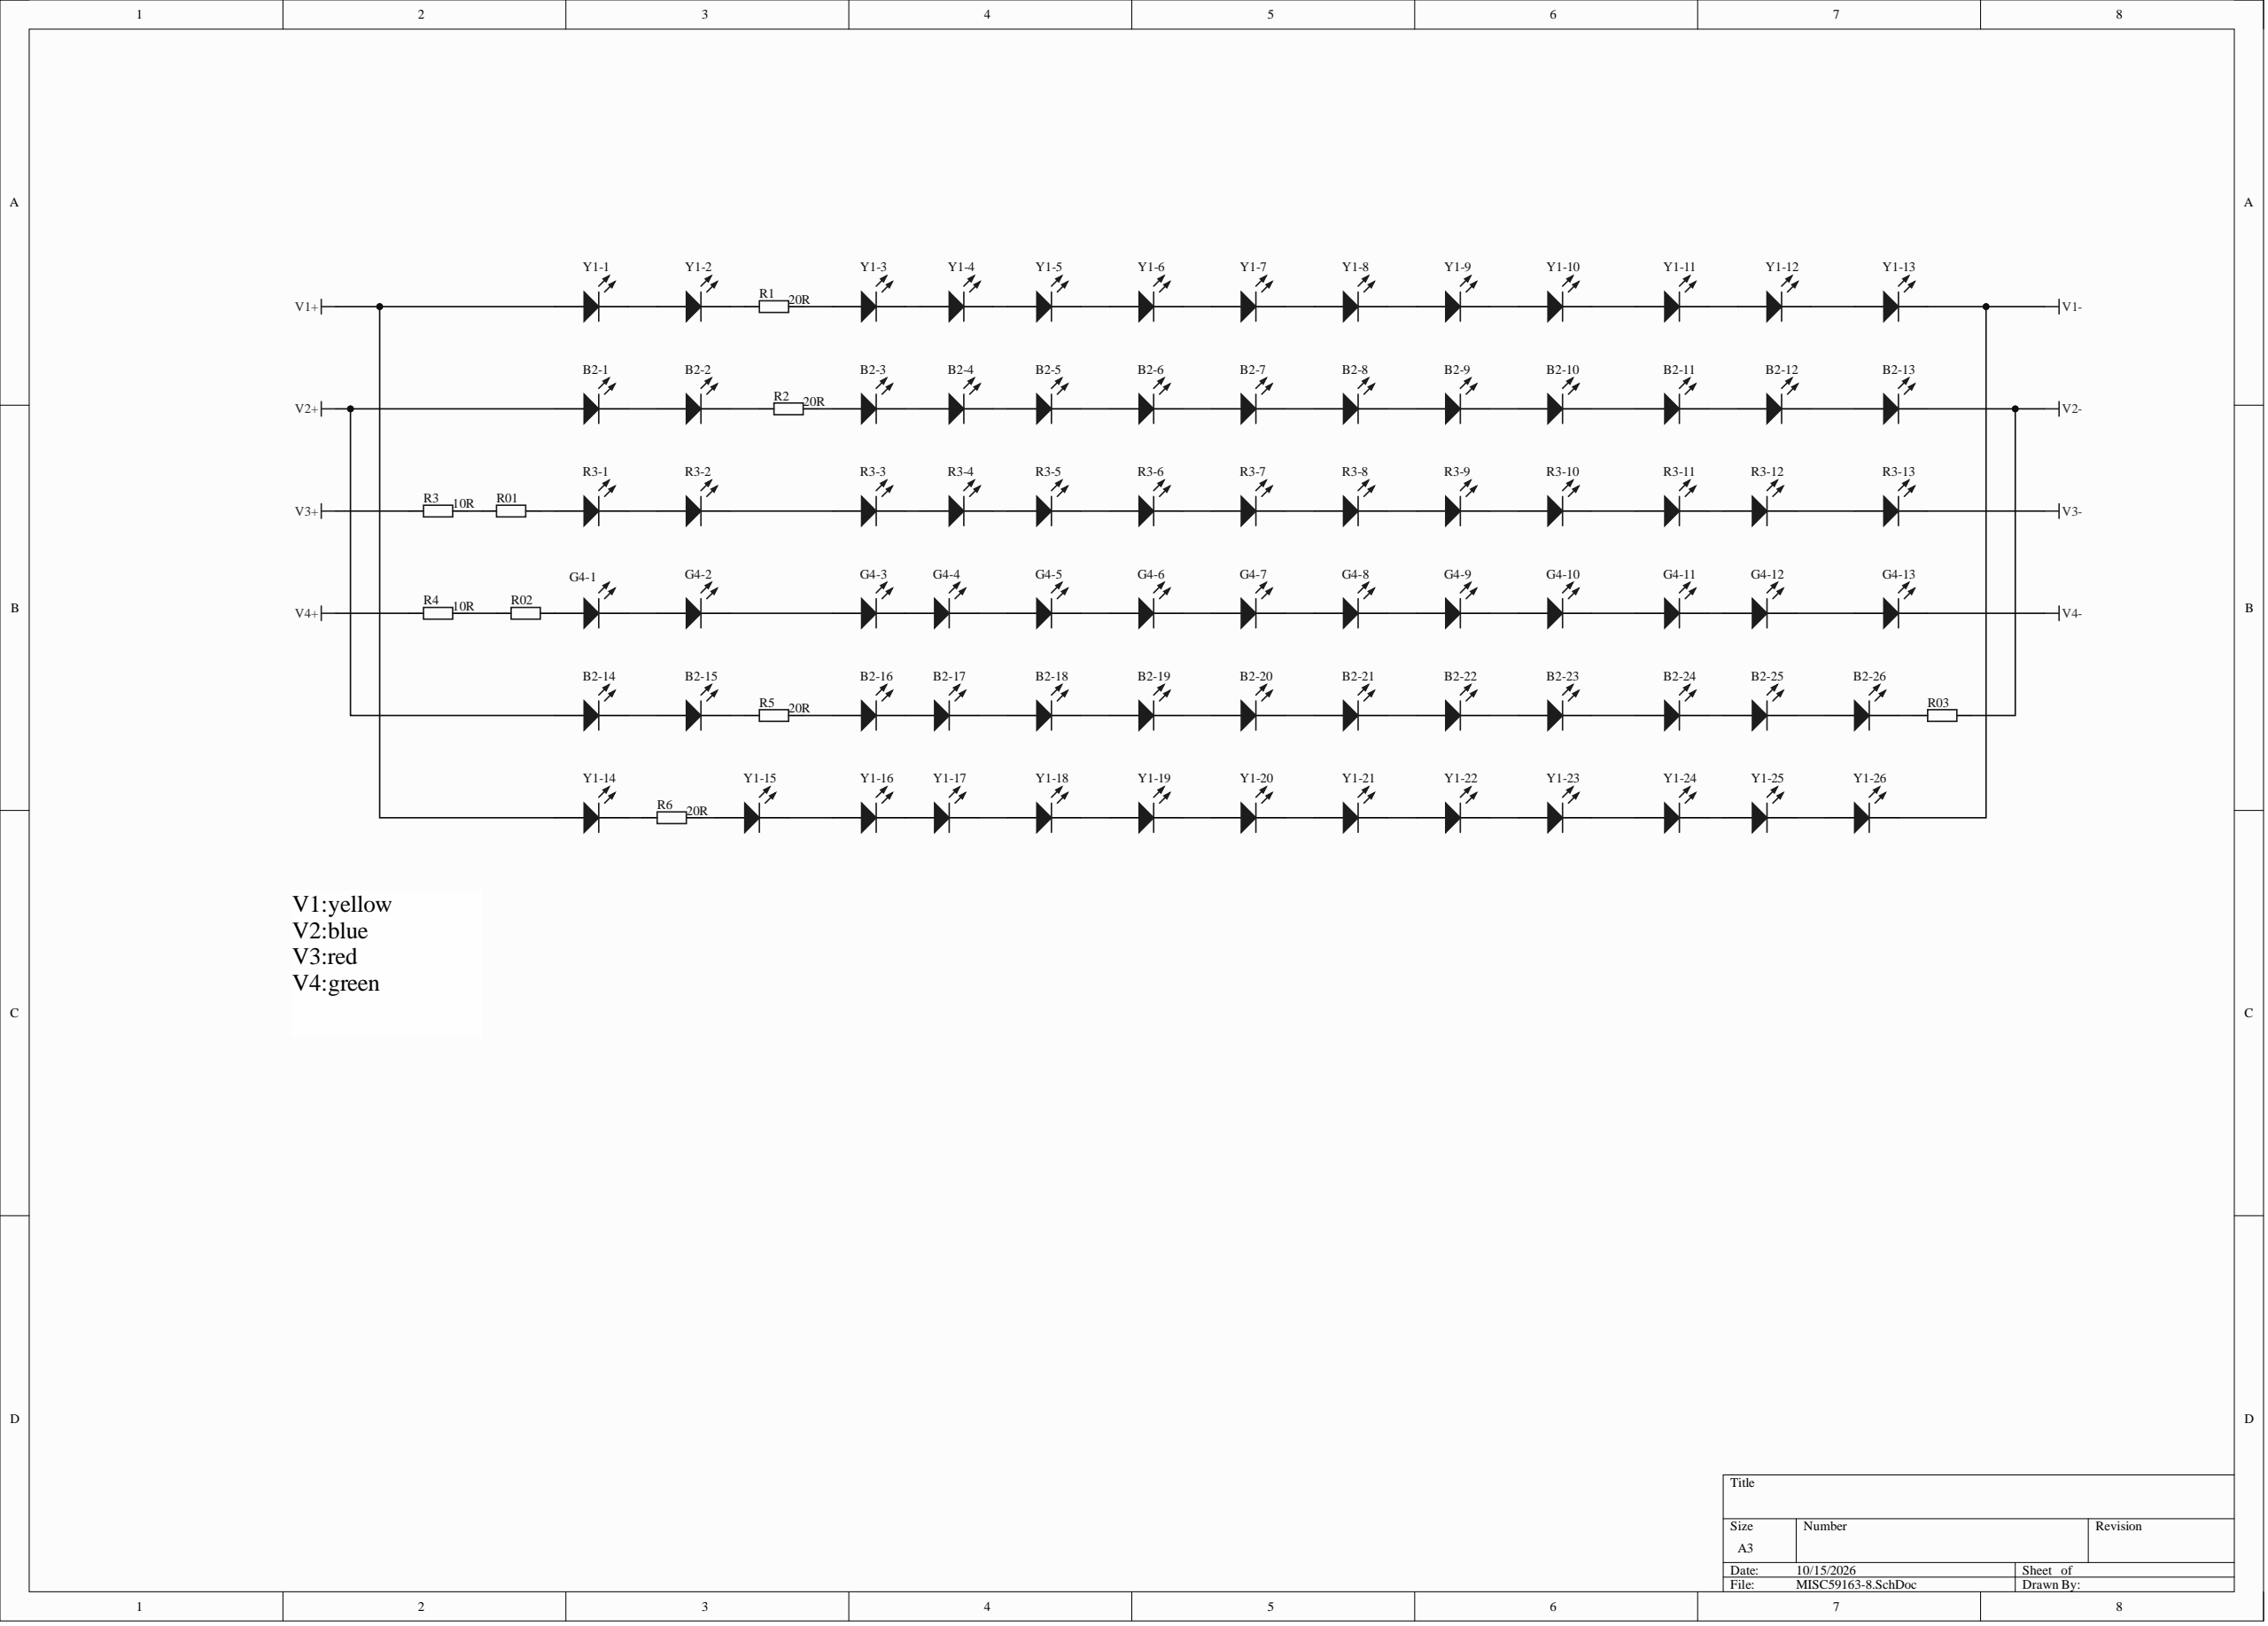Circuit board | Altium Designer | 87 parts | 85 nets
Bill of materials:
Comment,Description,Designator,Footprint,LibRef,Quantity
"2835A03-480B05-1S-F8","2835A03-480B05-1S-F8","B2-1, B2-2, B2-3, B2-4, B2-5, B2-6, B2-7, B2-8, B2-9, B2-10, B2-11, B2-12, B2-13","2835LED带透镜","LED2","13"
"2835A03-480B05-1S-F8","2835A03-480B05-1S-F8","B2-14, B2-15, B2-16, B2-17, B2-18, B2-19, B2-20, B2-21, B2-22, B2-23, B2-24, B2-25, B2-26","2835LED带透镜2","LED2","13"
"2835A03-525G05-2P-F10","2835A03-525G05-2P-F10","G4-1, G4-2, G4-3, G4-4, G4-5, G4-6, G4-7, G4-8, G4-9, G4-10, G4-11, G4-12","2835LED带透镜3","LED2","12"
"2835A03-525G05-2P-F10","2835A03-525G05-2P-F10","G4-13","2835LED带透镜2","LED2","1"
"jumper","QM8.2-D01  silver","R01, R02","贴片跳线QM8.2-D01","Res2","2"
"20O","0805 chip resistor","R1, R2, R5, R6","R0805","Res2","4"
"jumper","QM52-D01  silver","R03","贴片跳线","Res2","1"
"2835A03-630R05-2P-F10","2835A03-630R05-2P-F10","R3-1, R3-2, R3-3, R3-4, R3-5, R3-6, R3-7, R3-8, R3-9, R3-10, R3-11, R3-12, R3-13","2835LED带透镜3","LED2","13"
"10O","0805 chip resistor","R3, R4","R0805","Res2","2"
"2835A03-585Y05-2P-F10","2835A03-585Y05-2P-F10","Y1-1","2835LED带透镜1","LED2","1"
"2835A03-585Y05-2P-F10","2835A03-585Y05-2P-F10","Y1-2, Y1-3, Y1-4, Y1-5, Y1-6, Y1-7, Y1-8, Y1-9, Y1-10, Y1-11, Y1-12, Y1-13","2835LED带透镜","LED2","12"
"2835A03-585Y05-2P-F10","2835A03-585Y05-2P-F10","Y1-14, Y1-15, Y1-16, Y1-17, Y1-18, Y1-19, Y1-20, Y1-21, Y1-22, Y1-23, Y1-24, Y1-25, Y1-26","2835LED带透镜2","LED2","13"
Netlist (Protel format):
[
B2-1
2835LED带透镜
2835A03-480B05-1S-F8



]
[
B2-2
2835LED带透镜
2835A03-480B05-1S-F8



]
[
B2-3
2835LED带透镜
2835A03-480B05-1S-F8



]
[
B2-4
2835LED带透镜
2835A03-480B05-1S-F8



]
[
B2-5
2835LED带透镜
2835A03-480B05-1S-F8



]
[
B2-6
2835LED带透镜
2835A03-480B05-1S-F8



]
[
B2-7
2835LED带透镜
2835A03-480B05-1S-F8



]
[
B2-8
2835LED带透镜
2835A03-480B05-1S-F8



]
[
B2-9
2835LED带透镜
2835A03-480B05-1S-F8



]
[
B2-10
2835LED带透镜
2835A03-480B05-1S-F8



]
[
B2-11
2835LED带透镜
2835A03-480B05-1S-F8



]
[
B2-12
2835LED带透镜
2835A03-480B05-1S-F8



]
[
B2-13
2835LED带透镜
2835A03-480B05-1S-F8



]
[
B2-14
2835LED带透镜2
2835A03-480B05-1S-F8



]
[
B2-15
2835LED带透镜2
2835A03-480B05-1S-F8



]
[
B2-16
2835LED带透镜2
2835A03-480B05-1S-F8



]
[
B2-17
2835LED带透镜2
2835A03-480B05-1S-F8



]
[
B2-18
2835LED带透镜2
2835A03-480B05-1S-F8



]
[
B2-19
2835LED带透镜2
2835A03-480B05-1S-F8



]
[
B2-20
2835LED带透镜2
2835A03-480B05-1S-F8



]
[
B2-21
2835LED带透镜2
2835A03-480B05-1S-F8



]
[
B2-22
2835LED带透镜2
2835A03-480B05-1S-F8



]
[
B2-23
2835LED带透镜2
2835A03-480B05-1S-F8



]
[
B2-24
2835LED带透镜2
2835A03-480B05-1S-F8



]
[
B2-25
2835LED带透镜2
2835A03-480B05-1S-F8



]
[
B2-26
2835LED带透镜2
2835A03-480B05-1S-F8



]
[
G4-1
2835LED带透镜3
2835A03-525G05-2P-F10



]
[
G4-2
2835LED带透镜3
2835A03-525G05-2P-F10



]
[
G4-3
2835LED带透镜3
2835A03-525G05-2P-F10



]
[
G4-4
2835LED带透镜3
2835A03-525G05-2P-F10



]
[
G4-5
2835LED带透镜3
2835A03-525G05-2P-F10



]
[
G4-6
2835LED带透镜3
2835A03-525G05-2P-F10



]
[
G4-7
2835LED带透镜3
2835A03-525G05-2P-F10



]
[
G4-8
2835LED带透镜3
2835A03-525G05-2P-F10



]
[
G4-9
2835LED带透镜3
2835A03-525G05-2P-F10



]
[
G4-10
2835LED带透镜3
2835A03-525G05-2P-F10



]
[
G4-11
2835LED带透镜3
2835A03-525G05-2P-F10



]
[
G4-12
2835LED带透镜3
2835A03-525G05-2P-F10



]
[
G4-13
2835LED带透镜2
2835A03-525G05-2P-F10



]
[
R1
R0805
20O



]
[
R01
贴片跳线QM8.2-D01
jumper



]
[
R2
R0805
20O



]
[
R02
贴片跳线QM8.2-D01
jumper



]
[
R3
R0805
10O



]
[
R03
贴片跳线
jumper



]
[
R3-1
2835LED带透镜3
2835A03-630R05-2P-F10



]
[
R3-2
2835LED带透镜3
2835A03-630R05-2P-F10



]
[
R3-3
2835LED带透镜3
2835A03-630R05-2P-F10



]
[
R3-4
2835LED带透镜3
2835A03-630R05-2P-F10



]
[
R3-5
2835LED带透镜3
2835A03-630R05-2P-F10



]
[
R3-6
2835LED带透镜3
2835A03-630R05-2P-F10



]
[
R3-7
2835LED带透镜3
2835A03-630R05-2P-F10



]
[
R3-8
2835LED带透镜3
2835A03-630R05-2P-F10



]
[
R3-9
2835LED带透镜3
2835A03-630R05-2P-F10



]
[
R3-10
2835LED带透镜3
2835A03-630R05-2P-F10



]
[
R3-11
2835LED带透镜3
2835A03-630R05-2P-F10



]
[
R3-12
2835LED带透镜3
2835A03-630R05-2P-F10



]
[
R3-13
2835LED带透镜3
2835A03-630R05-2P-F10



]
[
R4
R0805
10O



]
[
R5
R0805
20O



]
[
R6
R0805
20O



]
[
Y1-1
2835LED带透镜1
2835A03-585Y05-2P-F10



]
[
Y1-2
2835LED带透镜
2835A03-585Y05-2P-F10



]
[
Y1-3
2835LED带透镜
2835A03-585Y05-2P-F10



]
[
Y1-4
2835LED带透镜
2835A03-585Y05-2P-F10



]
[
Y1-5
2835LED带透镜
2835A03-585Y05-2P-F10



]
[
Y1-6
2835LED带透镜
2835A03-585Y05-2P-F10



]
[
Y1-7
2835LED带透镜
2835A03-585Y05-2P-F10



]
[
Y1-8
2835LED带透镜
2835A03-585Y05-2P-F10



]
[
Y1-9
2835LED带透镜
2835A03-585Y05-2P-F10



]
[
Y1-10
2835LED带透镜
2835A03-585Y05-2P-F10



]
[
Y1-11
2835LED带透镜
2835A03-585Y05-2P-F10



]
[
Y1-12
2835LED带透镜
2835A03-585Y05-2P-F10



]
[
Y1-13
2835LED带透镜
2835A03-585Y05-2P-F10



]
[
Y1-14
2835LED带透镜2
2835A03-585Y05-2P-F10



]
[
Y1-15
2835LED带透镜2
2835A03-585Y05-2P-F10



]
[
Y1-16
2835LED带透镜2
2835A03-585Y05-2P-F10



]
[
Y1-17
2835LED带透镜2
2835A03-585Y05-2P-F10



]
[
Y1-18
2835LED带透镜2
2835A03-585Y05-2P-F10



]
[
Y1-19
2835LED带透镜2
2835A03-585Y05-2P-F10



]
[
Y1-20
2835LED带透镜2
2835A03-585Y05-2P-F10



]
[
Y1-21
2835LED带透镜2
2835A03-585Y05-2P-F10



]
[
Y1-22
2835LED带透镜2
2835A03-585Y05-2P-F10



]
[
Y1-23
2835LED带透镜2
2835A03-585Y05-2P-F10



]
[
Y1-24
2835LED带透镜2
2835A03-585Y05-2P-F10



]
[
Y1-25
2835LED带透镜2
2835A03-585Y05-2P-F10



]
[
Y1-26
2835LED带透镜2
2835A03-585Y05-2P-F10



]
(
V2-
B2-13-2
R03-2
)
(
V2+
B2-1-1
B2-14-1
)
(
V1-
Y1-13-2
Y1-26-2
)
(
V1+
Y1-1-1
Y1-14-1
)
(
NetY1-25_2
Y1-25-2
Y1-26-1
)
(
NetY1-24_2
Y1-24-2
Y1-25-1
)
(
NetY1-23_2
Y1-23-2
Y1-24-1
)
(
NetY1-22_2
Y1-22-2
Y1-23-1
)
(
NetY1-21_2
Y1-21-2
Y1-22-1
)
(
NetY1-20_2
Y1-20-2
Y1-21-1
)
(
NetY1-19_2
Y1-19-2
Y1-20-1
)
(
NetY1-18_2
Y1-18-2
Y1-19-1
)
(
NetY1-17_2
Y1-17-2
Y1-18-1
)
(
NetY1-16_2
Y1-16-2
Y1-17-1
)
(
NetY1-15_2
Y1-15-2
Y1-16-1
)
(
NetY1-12_2
Y1-12-2
Y1-13-1
)
(
NetY1-11_2
Y1-11-2
Y1-12-1
)
(
NetY1-10_2
Y1-10-2
Y1-11-1
)
(
NetY1-9_2
Y1-9-2
Y1-10-1
)
(
NetY1-8_2
Y1-8-2
Y1-9-1
)
(
NetY1-7_2
Y1-7-2
Y1-8-1
)
(
NetY1-6_2
Y1-6-2
Y1-7-1
)
(
NetY1-5_2
Y1-5-2
Y1-6-1
)
(
NetY1-4_2
Y1-4-2
Y1-5-1
)
(
NetY1-3_2
Y1-3-2
Y1-4-1
)
(
NetY1-1_2
Y1-1-2
Y1-2-1
)
(
NetR6_2
R6-2
Y1-15-1
)
(
NetR6_1
R6-1
Y1-14-2
)
(
NetR3-12_1
R3-12-1
R3-13-2
)
(
NetR3-11_1
R3-11-1
R3-12-2
)
(
NetR3-10_1
R3-10-1
R3-11-2
)
(
NetR3-9_1
R3-9-1
R3-10-2
)
(
NetR3-8_1
R3-8-1
R3-9-2
)
(
NetR3-7_1
R3-7-1
R3-8-2
)
(
NetR3-6_1
R3-6-1
R3-7-2
)
(
NetR3-5_1
R3-5-1
R3-6-2
)
(
NetR3-4_1
R3-4-1
R3-5-2
)
(
NetR3-3_1
R3-3-1
R3-4-2
)
(
NetR3-2_1
R3-2-1
R3-3-2
)
(
NetR3-1_1
R3-1-1
R3-2-2
)
(
NetR02_1
R02-1
R4-2
)
(
NetR01_2
R01-2
R3-1-2
)
(
NetR1_2
R1-2
Y1-3-1
)
(
NetR01_1
R01-1
R3-2
)
(
NetR1_1
R1-1
Y1-2-2
)
(
NetG4-12_2
G4-12-2
G4-13-1
)
(
NetG4-11_2
G4-11-2
G4-12-1
)
(
NetG4-10_2
G4-10-2
G4-11-1
)
(
NetG4-9_2
G4-9-2
G4-10-1
)
(
NetG4-8_2
G4-8-2
G4-9-1
)
(
NetG4-7_2
G4-7-2
G4-8-1
)
(
NetG4-6_2
G4-6-2
G4-7-1
)
(
NetG4-5_2
G4-5-2
G4-6-1
)
(
NetG4-4_2
G4-4-2
G4-5-1
)
(
NetG4-3_2
G4-3-2
G4-4-1
)
(
NetG4-2_2
G4-2-2
G4-3-1
)
(
NetG4-1_2
G4-1-2
G4-2-1
)
(
NetG4-1_1
G4-1-1
R02-2
)
(
NetB2-26_2
B2-26-2
R03-1
)
(
NetB2-25_2
B2-25-2
B2-26-1
)
(
NetB2-24_2
B2-24-2
B2-25-1
)
(
NetB2-23_2
B2-23-2
B2-24-1
)
(
NetB2-22_2
B2-22-2
B2-23-1
)
(
NetB2-21_2
B2-21-2
B2-22-1
)
(
NetB2-20_2
B2-20-2
B2-21-1
)
(
NetB2-19_2
B2-19-2
B2-20-1
)
(
NetB2-18_2
B2-18-2
B2-19-1
)
(
NetB2-17_2
B2-17-2
B2-18-1
)
(
NetB2-16_2
B2-16-2
B2-17-1
)
(
NetB2-16_1
B2-16-1
R5-2
)
(
NetB2-15_2
B2-15-2
R5-1
)
(
NetB2-14_2
B2-14-2
B2-15-1
)
(
NetB2-12_2
B2-12-2
B2-13-1
)
(
NetB2-11_2
B2-11-2
B2-12-1
)
(
NetB2-10_2
B2-10-2
B2-11-1
)
(
NetB2-9_2
B2-9-2
B2-10-1
)
(
NetB2-8_2
B2-8-2
B2-9-1
)
(
NetB2-7_2
B2-7-2
B2-8-1
)
(
NetB2-6_2
B2-6-2
B2-7-1
)
(
NetB2-5_2
B2-5-2
B2-6-1
)
(
NetB2-4_2
B2-4-2
B2-5-1
)
(
NetB2-3_2
B2-3-2
B2-4-1
)
(
NetB2-3_1
B2-3-1
R2-2
)
(
NetB2-2_2
B2-2-2
R2-1
)
(
NetB2-1_2
B2-1-2
B2-2-1
)